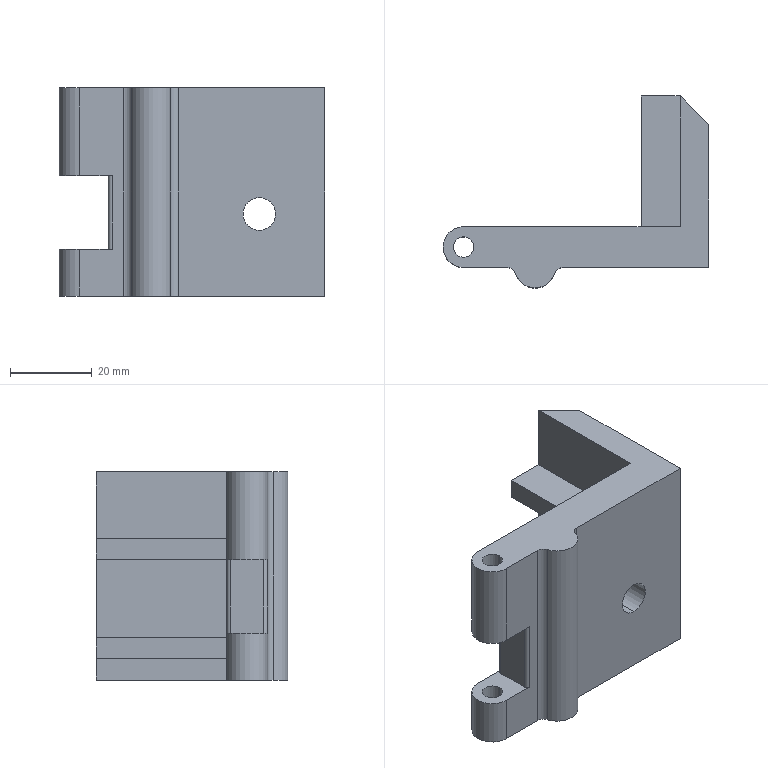Part | Creo | features CURVE 7, PROTRUSION 5, DATUM PLANE 3, ROUND 3, CUT 2, CHAMFER 1, COORDINATE SYSTEM 1 | 1 solid | 34 faces | box 65 x 47 x 51 mm | volume 44748 mm3 | plane 21 | cylinder 13 | commonest cylinder face diameters 5 x4 10 x3 2 x2 4 x2 8 x2
STEP:
#1=CARTESIAN_POINT('',(0.,0.,0.));
#2=DIRECTION('',(0.,0.,1.));
#3=DIRECTION('',(1.,0.,0.));
#4=AXIS2_PLACEMENT_3D('',#1,#2,#3);
#5=CARTESIAN_POINT('',(28.,42.,-20.5));
#6=VERTEX_POINT('',#5);
#7=CARTESIAN_POINT('',(35.,35.,-20.5));
#8=VERTEX_POINT('',#7);
#9=CARTESIAN_POINT('',(28.,42.,-20.5));
#10=DIRECTION('',(0.7071,-0.7071,0.));
#11=VECTOR('',#10,9.899);
#12=LINE('',#9,#11);
#13=EDGE_CURVE('',#6,#8,#12,.T.);
#14=ORIENTED_EDGE('',*,*,#13,.F.);
#15=CARTESIAN_POINT('',(28.,10.,-20.5));
#16=VERTEX_POINT('',#15);
#17=CARTESIAN_POINT('',(28.,42.,-20.5));
#18=DIRECTION('',(0.,-1.,0.));
#19=VECTOR('',#18,32.);
#20=LINE('',#17,#19);
#21=EDGE_CURVE('',#6,#16,#20,.T.);
#22=ORIENTED_EDGE('',*,*,#21,.T.);
#23=CARTESIAN_POINT('',(-25.,10.,-20.5));
#24=VERTEX_POINT('',#23);
#25=CARTESIAN_POINT('',(28.,10.,-20.5));
#26=DIRECTION('',(-1.,0.,0.));
#27=VECTOR('',#26,53.);
#28=LINE('',#25,#27);
#29=EDGE_CURVE('',#16,#24,#28,.T.);
#30=ORIENTED_EDGE('',*,*,#29,.T.);
#31=CARTESIAN_POINT('',(-25.,0.,-20.5));
#32=VERTEX_POINT('',#31);
#33=CARTESIAN_POINT('',(-25.,5.,-20.5));
#34=DIRECTION('',(0.,0.,1.));
#35=DIRECTION('',(0.,1.,0.));
#36=AXIS2_PLACEMENT_3D('',#33,#34,#35);
#37=CIRCLE('',#36,5.);
#38=EDGE_CURVE('',#24,#32,#37,.T.);
#39=ORIENTED_EDGE('',*,*,#38,.T.);
#40=CARTESIAN_POINT('',(-14.208,0.,-20.5));
#41=VERTEX_POINT('',#40);
#42=CARTESIAN_POINT('',(-25.,0.,-20.5));
#43=DIRECTION('',(1.,0.,0.));
#44=VECTOR('',#43,10.792);
#45=LINE('',#42,#44);
#46=EDGE_CURVE('',#32,#41,#45,.T.);
#47=ORIENTED_EDGE('',*,*,#46,.T.);
#48=CARTESIAN_POINT('',(-12.292,-1.429,-20.5));
#49=VERTEX_POINT('',#48);
#50=CARTESIAN_POINT('',(-14.208,-2.,-20.5));
#51=DIRECTION('',(0.,0.,1.));
#52=DIRECTION('',(0.9583,0.2857,0.));
#53=AXIS2_PLACEMENT_3D('',#50,#51,#52);
#54=CIRCLE('',#53,2.);
#55=EDGE_CURVE('',#49,#41,#54,.T.);
#56=ORIENTED_EDGE('',*,*,#55,.F.);
#57=CARTESIAN_POINT('',(-2.708,-1.429,-20.5));
#58=VERTEX_POINT('',#57);
#59=CARTESIAN_POINT('',(-7.5,0.,-20.5));
#60=DIRECTION('',(0.,0.,-1.));
#61=DIRECTION('',(0.9583,-0.2857,0.));
#62=AXIS2_PLACEMENT_3D('',#59,#60,#61);
#63=CIRCLE('',#62,5.);
#64=EDGE_CURVE('',#58,#49,#63,.T.);
#65=ORIENTED_EDGE('',*,*,#64,.F.);
#66=CARTESIAN_POINT('',(-0.7918,0.,-20.5));
#67=VERTEX_POINT('',#66);
#68=CARTESIAN_POINT('',(-0.7918,-2.,-20.5));
#69=DIRECTION('',(0.,0.,1.));
#70=DIRECTION('',(0.,1.,0.));
#71=AXIS2_PLACEMENT_3D('',#68,#69,#70);
#72=CIRCLE('',#71,2.);
#73=EDGE_CURVE('',#67,#58,#72,.T.);
#74=ORIENTED_EDGE('',*,*,#73,.F.);
#75=CARTESIAN_POINT('',(35.,0.,-20.5));
#76=VERTEX_POINT('',#75);
#77=CARTESIAN_POINT('',(35.,0.,-20.5));
#78=DIRECTION('',(-1.,0.,0.));
#79=VECTOR('',#78,35.792);
#80=LINE('',#77,#79);
#81=EDGE_CURVE('',#76,#67,#80,.T.);
#82=ORIENTED_EDGE('',*,*,#81,.F.);
#83=CARTESIAN_POINT('',(35.,0.,-20.5));
#84=DIRECTION('',(0.,1.,0.));
#85=VECTOR('',#84,35.);
#86=LINE('',#83,#85);
#87=EDGE_CURVE('',#76,#8,#86,.T.);
#88=ORIENTED_EDGE('',*,*,#87,.T.);
#89=EDGE_LOOP('',(#14,#22,#30,#39,#47,#56,#65,#74,#82,#88));
#90=FACE_OUTER_BOUND('',#89,.F.);
#91=CARTESIAN_POINT('',(-22.5,5.,-20.5));
#92=VERTEX_POINT('',#91);
#93=CARTESIAN_POINT('',(-27.5,5.,-20.5));
#94=VERTEX_POINT('',#93);
#95=CARTESIAN_POINT('',(-25.,5.,-20.5));
#96=DIRECTION('',(0.,0.,-1.));
#97=DIRECTION('',(1.,0.,0.));
#98=AXIS2_PLACEMENT_3D('',#95,#96,#97);
#99=CIRCLE('',#98,2.5);
#100=EDGE_CURVE('',#92,#94,#99,.T.);
#101=ORIENTED_EDGE('',*,*,#100,.T.);
#102=CARTESIAN_POINT('',(-25.,5.,-20.5));
#103=DIRECTION('',(0.,0.,-1.));
#104=DIRECTION('',(-1.,0.,0.));
#105=AXIS2_PLACEMENT_3D('',#102,#103,#104);
#106=CIRCLE('',#105,2.5);
#107=EDGE_CURVE('',#94,#92,#106,.T.);
#108=ORIENTED_EDGE('',*,*,#107,.T.);
#109=EDGE_LOOP('',(#101,#108));
#110=FACE_BOUND('',#109,.F.);
#111=CARTESIAN_POINT('',(0.,0.,-20.5));
#112=DIRECTION('',(0.,0.,1.));
#113=DIRECTION('',(1.,0.,0.));
#114=AXIS2_PLACEMENT_3D('',#111,#112,#113);
#115=PLANE('',#114);
#116=ADVANCED_FACE('',(#90,#110),#115,.F.);
#117=CARTESIAN_POINT('',(-27.5,5.,-9.));
#118=VERTEX_POINT('',#117);
#119=CARTESIAN_POINT('',(-22.5,5.,-9.));
#120=VERTEX_POINT('',#119);
#121=CARTESIAN_POINT('',(-25.,5.,-9.));
#122=DIRECTION('',(0.,0.,1.));
#123=DIRECTION('',(-1.,0.,0.));
#124=AXIS2_PLACEMENT_3D('',#121,#122,#123);
#125=CIRCLE('',#124,2.5);
#126=EDGE_CURVE('',#118,#120,#125,.T.);
#127=ORIENTED_EDGE('',*,*,#126,.F.);
#128=CARTESIAN_POINT('',(-27.5,5.,-20.5));
#129=DIRECTION('',(0.,0.,1.));
#130=VECTOR('',#129,11.5);
#131=LINE('',#128,#130);
#132=EDGE_CURVE('',#94,#118,#131,.T.);
#133=ORIENTED_EDGE('',*,*,#132,.F.);
#134=ORIENTED_EDGE('',*,*,#100,.F.);
#135=CARTESIAN_POINT('',(-22.5,5.,-20.5));
#136=DIRECTION('',(0.,0.,1.));
#137=VECTOR('',#136,11.5);
#138=LINE('',#135,#137);
#139=EDGE_CURVE('',#92,#120,#138,.T.);
#140=ORIENTED_EDGE('',*,*,#139,.T.);
#141=EDGE_LOOP('',(#127,#133,#134,#140));
#142=FACE_OUTER_BOUND('',#141,.F.);
#143=CARTESIAN_POINT('',(-25.,5.,-20.5));
#144=DIRECTION('',(0.,0.,1.));
#145=DIRECTION('',(1.,0.,0.));
#146=AXIS2_PLACEMENT_3D('',#143,#144,#145);
#147=CYLINDRICAL_SURFACE('',#146,2.5);
#148=ADVANCED_FACE('',(#142),#147,.F.);
#149=CARTESIAN_POINT('',(-22.5,5.,30.5));
#150=VERTEX_POINT('',#149);
#151=CARTESIAN_POINT('',(-22.5,5.,9.));
#152=VERTEX_POINT('',#151);
#153=CARTESIAN_POINT('',(-22.5,5.,30.5));
#154=DIRECTION('',(0.,0.,-1.));
#155=VECTOR('',#154,21.5);
#156=LINE('',#153,#155);
#157=EDGE_CURVE('',#150,#152,#156,.T.);
#158=ORIENTED_EDGE('',*,*,#157,.F.);
#159=CARTESIAN_POINT('',(-27.5,5.,30.5));
#160=VERTEX_POINT('',#159);
#161=CARTESIAN_POINT('',(-25.,5.,30.5));
#162=DIRECTION('',(0.,0.,-1.));
#163=DIRECTION('',(1.,0.,0.));
#164=AXIS2_PLACEMENT_3D('',#161,#162,#163);
#165=CIRCLE('',#164,2.5);
#166=EDGE_CURVE('',#150,#160,#165,.T.);
#167=ORIENTED_EDGE('',*,*,#166,.T.);
#168=CARTESIAN_POINT('',(-27.5,5.,9.));
#169=VERTEX_POINT('',#168);
#170=CARTESIAN_POINT('',(-27.5,5.,9.));
#171=DIRECTION('',(0.,0.,1.));
#172=VECTOR('',#171,21.5);
#173=LINE('',#170,#172);
#174=EDGE_CURVE('',#169,#160,#173,.T.);
#175=ORIENTED_EDGE('',*,*,#174,.F.);
#176=CARTESIAN_POINT('',(-25.,5.,9.));
#177=DIRECTION('',(0.,0.,1.));
#178=DIRECTION('',(-1.,0.,0.));
#179=AXIS2_PLACEMENT_3D('',#176,#177,#178);
#180=CIRCLE('',#179,2.5);
#181=EDGE_CURVE('',#169,#152,#180,.T.);
#182=ORIENTED_EDGE('',*,*,#181,.T.);
#183=EDGE_LOOP('',(#158,#167,#175,#182));
#184=FACE_OUTER_BOUND('',#183,.F.);
#185=CARTESIAN_POINT('',(-25.,5.,-20.5));
#186=DIRECTION('',(0.,0.,1.));
#187=DIRECTION('',(1.,0.,0.));
#188=AXIS2_PLACEMENT_3D('',#185,#186,#187);
#189=CYLINDRICAL_SURFACE('',#188,2.5);
#190=ADVANCED_FACE('',(#184),#189,.F.);
#191=CARTESIAN_POINT('',(-18.,9.,-9.));
#192=VERTEX_POINT('',#191);
#193=CARTESIAN_POINT('',(-18.,1.,-9.));
#194=VERTEX_POINT('',#193);
#195=CARTESIAN_POINT('',(-18.,9.,-9.));
#196=DIRECTION('',(0.,-1.,0.));
#197=VECTOR('',#196,8.);
#198=LINE('',#195,#197);
#199=EDGE_CURVE('',#192,#194,#198,.T.);
#200=ORIENTED_EDGE('',*,*,#199,.T.);
#201=CARTESIAN_POINT('',(-17.,0.,-9.));
#202=VERTEX_POINT('',#201);
#203=CARTESIAN_POINT('',(-17.,1.,-9.));
#204=DIRECTION('',(0.,0.,-1.));
#205=DIRECTION('',(0.,-1.,0.));
#206=AXIS2_PLACEMENT_3D('',#203,#204,#205);
#207=CIRCLE('',#206,1.);
#208=EDGE_CURVE('',#202,#194,#207,.T.);
#209=ORIENTED_EDGE('',*,*,#208,.F.);
#210=CARTESIAN_POINT('',(-25.,0.,-9.));
#211=VERTEX_POINT('',#210);
#212=CARTESIAN_POINT('',(-17.,0.,-9.));
#213=DIRECTION('',(-1.,0.,0.));
#214=VECTOR('',#213,8.);
#215=LINE('',#212,#214);
#216=EDGE_CURVE('',#202,#211,#215,.T.);
#217=ORIENTED_EDGE('',*,*,#216,.T.);
#218=CARTESIAN_POINT('',(-25.,10.,-9.));
#219=VERTEX_POINT('',#218);
#220=CARTESIAN_POINT('',(-25.,5.,-9.));
#221=DIRECTION('',(0.,0.,-1.));
#222=DIRECTION('',(0.,-1.,0.));
#223=AXIS2_PLACEMENT_3D('',#220,#221,#222);
#224=CIRCLE('',#223,5.);
#225=EDGE_CURVE('',#211,#219,#224,.T.);
#226=ORIENTED_EDGE('',*,*,#225,.T.);
#227=CARTESIAN_POINT('',(-17.,10.,-9.));
#228=VERTEX_POINT('',#227);
#229=CARTESIAN_POINT('',(-25.,10.,-9.));
#230=DIRECTION('',(1.,0.,0.));
#231=VECTOR('',#230,8.);
#232=LINE('',#229,#231);
#233=EDGE_CURVE('',#219,#228,#232,.T.);
#234=ORIENTED_EDGE('',*,*,#233,.T.);
#235=CARTESIAN_POINT('',(-17.,9.,-9.));
#236=DIRECTION('',(0.,0.,-1.));
#237=DIRECTION('',(-1.,0.,0.));
#238=AXIS2_PLACEMENT_3D('',#235,#236,#237);
#239=CIRCLE('',#238,1.);
#240=EDGE_CURVE('',#192,#228,#239,.T.);
#241=ORIENTED_EDGE('',*,*,#240,.F.);
#242=EDGE_LOOP('',(#200,#209,#217,#226,#234,#241));
#243=FACE_OUTER_BOUND('',#242,.F.);
#244=ORIENTED_EDGE('',*,*,#126,.T.);
#245=CARTESIAN_POINT('',(-25.,5.,-9.));
#246=DIRECTION('',(0.,0.,1.));
#247=DIRECTION('',(1.,0.,0.));
#248=AXIS2_PLACEMENT_3D('',#245,#246,#247);
#249=CIRCLE('',#248,2.5);
#250=EDGE_CURVE('',#120,#118,#249,.T.);
#251=ORIENTED_EDGE('',*,*,#250,.T.);
#252=EDGE_LOOP('',(#244,#251));
#253=FACE_BOUND('',#252,.F.);
#254=CARTESIAN_POINT('',(-18.,10.,-9.));
#255=DIRECTION('',(0.,0.,-1.));
#256=DIRECTION('',(-1.,0.,0.));
#257=AXIS2_PLACEMENT_3D('',#254,#255,#256);
#258=PLANE('',#257);
#259=ADVANCED_FACE('',(#243,#253),#258,.F.);
#260=ORIENTED_EDGE('',*,*,#250,.F.);
#261=ORIENTED_EDGE('',*,*,#139,.F.);
#262=ORIENTED_EDGE('',*,*,#107,.F.);
#263=ORIENTED_EDGE('',*,*,#132,.T.);
#264=EDGE_LOOP('',(#260,#261,#262,#263));
#265=FACE_OUTER_BOUND('',#264,.F.);
#266=CARTESIAN_POINT('',(-25.,5.,-20.5));
#267=DIRECTION('',(0.,0.,1.));
#268=DIRECTION('',(1.,0.,0.));
#269=AXIS2_PLACEMENT_3D('',#266,#267,#268);
#270=CYLINDRICAL_SURFACE('',#269,2.5);
#271=ADVANCED_FACE('',(#265),#270,.F.);
#272=ORIENTED_EDGE('',*,*,#174,.T.);
#273=CARTESIAN_POINT('',(-25.,5.,30.5));
#274=DIRECTION('',(0.,0.,-1.));
#275=DIRECTION('',(-1.,0.,0.));
#276=AXIS2_PLACEMENT_3D('',#273,#274,#275);
#277=CIRCLE('',#276,2.5);
#278=EDGE_CURVE('',#160,#150,#277,.T.);
#279=ORIENTED_EDGE('',*,*,#278,.T.);
#280=ORIENTED_EDGE('',*,*,#157,.T.);
#281=CARTESIAN_POINT('',(-25.,5.,9.));
#282=DIRECTION('',(0.,0.,1.));
#283=DIRECTION('',(1.,0.,0.));
#284=AXIS2_PLACEMENT_3D('',#281,#282,#283);
#285=CIRCLE('',#284,2.5);
#286=EDGE_CURVE('',#152,#169,#285,.T.);
#287=ORIENTED_EDGE('',*,*,#286,.T.);
#288=EDGE_LOOP('',(#272,#279,#280,#287));
#289=FACE_OUTER_BOUND('',#288,.F.);
#290=CARTESIAN_POINT('',(-25.,5.,-20.5));
#291=DIRECTION('',(0.,0.,1.));
#292=DIRECTION('',(1.,0.,0.));
#293=AXIS2_PLACEMENT_3D('',#290,#291,#292);
#294=CYLINDRICAL_SURFACE('',#293,2.5);
#295=ADVANCED_FACE('',(#289),#294,.F.);
#296=CARTESIAN_POINT('',(35.,35.,30.5));
#297=VERTEX_POINT('',#296);
#298=CARTESIAN_POINT('',(28.,42.,30.5));
#299=VERTEX_POINT('',#298);
#300=CARTESIAN_POINT('',(35.,35.,30.5));
#301=DIRECTION('',(-0.7071,0.7071,0.));
#302=VECTOR('',#301,9.899);
#303=LINE('',#300,#302);
#304=EDGE_CURVE('',#297,#299,#303,.T.);
#305=ORIENTED_EDGE('',*,*,#304,.F.);
#306=CARTESIAN_POINT('',(35.,0.,30.5));
#307=VERTEX_POINT('',#306);
#308=CARTESIAN_POINT('',(35.,35.,30.5));
#309=DIRECTION('',(0.,-1.,0.));
#310=VECTOR('',#309,35.);
#311=LINE('',#308,#310);
#312=EDGE_CURVE('',#297,#307,#311,.T.);
#313=ORIENTED_EDGE('',*,*,#312,.T.);
#314=CARTESIAN_POINT('',(-0.7918,0.,30.5));
#315=VERTEX_POINT('',#314);
#316=CARTESIAN_POINT('',(-0.7918,0.,30.5));
#317=DIRECTION('',(1.,0.,0.));
#318=VECTOR('',#317,35.792);
#319=LINE('',#316,#318);
#320=EDGE_CURVE('',#315,#307,#319,.T.);
#321=ORIENTED_EDGE('',*,*,#320,.F.);
#322=CARTESIAN_POINT('',(-2.708,-1.429,30.5));
#323=VERTEX_POINT('',#322);
#324=CARTESIAN_POINT('',(-0.7918,-2.,30.5));
#325=DIRECTION('',(0.,0.,-1.));
#326=DIRECTION('',(-0.9583,0.2857,0.));
#327=AXIS2_PLACEMENT_3D('',#324,#325,#326);
#328=CIRCLE('',#327,2.);
#329=EDGE_CURVE('',#323,#315,#328,.T.);
#330=ORIENTED_EDGE('',*,*,#329,.F.);
#331=CARTESIAN_POINT('',(-12.292,-1.429,30.5));
#332=VERTEX_POINT('',#331);
#333=CARTESIAN_POINT('',(-7.5,0.,30.5));
#334=DIRECTION('',(0.,0.,1.));
#335=DIRECTION('',(-0.9583,-0.2857,0.));
#336=AXIS2_PLACEMENT_3D('',#333,#334,#335);
#337=CIRCLE('',#336,5.);
#338=EDGE_CURVE('',#332,#323,#337,.T.);
#339=ORIENTED_EDGE('',*,*,#338,.F.);
#340=CARTESIAN_POINT('',(-14.208,0.,30.5));
#341=VERTEX_POINT('',#340);
#342=CARTESIAN_POINT('',(-14.208,-2.,30.5));
#343=DIRECTION('',(0.,0.,-1.));
#344=DIRECTION('',(0.,1.,0.));
#345=AXIS2_PLACEMENT_3D('',#342,#343,#344);
#346=CIRCLE('',#345,2.);
#347=EDGE_CURVE('',#341,#332,#346,.T.);
#348=ORIENTED_EDGE('',*,*,#347,.F.);
#349=CARTESIAN_POINT('',(-25.,0.,30.5));
#350=VERTEX_POINT('',#349);
#351=CARTESIAN_POINT('',(-25.,0.,30.5));
#352=DIRECTION('',(1.,0.,0.));
#353=VECTOR('',#352,10.792);
#354=LINE('',#351,#353);
#355=EDGE_CURVE('',#350,#341,#354,.T.);
#356=ORIENTED_EDGE('',*,*,#355,.F.);
#357=CARTESIAN_POINT('',(-25.,10.,30.5));
#358=VERTEX_POINT('',#357);
#359=CARTESIAN_POINT('',(-25.,5.,30.5));
#360=DIRECTION('',(0.,0.,1.));
#361=DIRECTION('',(0.,1.,0.));
#362=AXIS2_PLACEMENT_3D('',#359,#360,#361);
#363=CIRCLE('',#362,5.);
#364=EDGE_CURVE('',#358,#350,#363,.T.);
#365=ORIENTED_EDGE('',*,*,#364,.F.);
#366=CARTESIAN_POINT('',(28.,10.,30.5));
#367=VERTEX_POINT('',#366);
#368=CARTESIAN_POINT('',(28.,10.,30.5));
#369=DIRECTION('',(-1.,0.,0.));
#370=VECTOR('',#369,53.);
#371=LINE('',#368,#370);
#372=EDGE_CURVE('',#367,#358,#371,.T.);
#373=ORIENTED_EDGE('',*,*,#372,.F.);
#374=CARTESIAN_POINT('',(28.,42.,30.5));
#375=DIRECTION('',(0.,-1.,0.));
#376=VECTOR('',#375,32.);
#377=LINE('',#374,#376);
#378=EDGE_CURVE('',#299,#367,#377,.T.);
#379=ORIENTED_EDGE('',*,*,#378,.F.);
#380=EDGE_LOOP('',(#305,#313,#321,#330,#339,#348,#356,#365,#373,#379));
#381=FACE_OUTER_BOUND('',#380,.F.);
#382=ORIENTED_EDGE('',*,*,#166,.F.);
#383=ORIENTED_EDGE('',*,*,#278,.F.);
#384=EDGE_LOOP('',(#382,#383));
#385=FACE_BOUND('',#384,.F.);
#386=CARTESIAN_POINT('',(0.,0.,30.5));
#387=DIRECTION('',(0.,0.,1.));
#388=DIRECTION('',(1.,0.,0.));
#389=AXIS2_PLACEMENT_3D('',#386,#387,#388);
#390=PLANE('',#389);
#391=ADVANCED_FACE('',(#381,#385),#390,.T.);
#392=ORIENTED_EDGE('',*,*,#304,.T.);
#393=CARTESIAN_POINT('',(28.,42.,14.13));
#394=VERTEX_POINT('',#393);
#395=CARTESIAN_POINT('',(28.,42.,14.13));
#396=DIRECTION('',(0.,0.,1.));
#397=VECTOR('',#396,16.37);
#398=LINE('',#395,#397);
#399=EDGE_CURVE('',#394,#299,#398,.T.);
#400=ORIENTED_EDGE('',*,*,#399,.F.);
#401=CARTESIAN_POINT('',(28.,42.,9.13));
#402=VERTEX_POINT('',#401);
#403=CARTESIAN_POINT('',(28.,42.,9.13));
#404=DIRECTION('',(0.,0.,1.));
#405=VECTOR('',#404,5.);
#406=LINE('',#403,#405);
#407=EDGE_CURVE('',#402,#394,#406,.T.);
#408=ORIENTED_EDGE('',*,*,#407,.F.);
#409=CARTESIAN_POINT('',(28.,42.,-10.13));
#410=VERTEX_POINT('',#409);
#411=CARTESIAN_POINT('',(28.,42.,-10.13));
#412=DIRECTION('',(0.,0.,1.));
#413=VECTOR('',#412,19.26);
#414=LINE('',#411,#413);
#415=EDGE_CURVE('',#410,#402,#414,.T.);
#416=ORIENTED_EDGE('',*,*,#415,.F.);
#417=CARTESIAN_POINT('',(28.,42.,-15.13));
#418=VERTEX_POINT('',#417);
#419=CARTESIAN_POINT('',(28.,42.,-15.13));
#420=DIRECTION('',(0.,0.,1.));
#421=VECTOR('',#420,5.);
#422=LINE('',#419,#421);
#423=EDGE_CURVE('',#418,#410,#422,.T.);
#424=ORIENTED_EDGE('',*,*,#423,.F.);
#425=CARTESIAN_POINT('',(28.,42.,-20.5));
#426=DIRECTION('',(0.,0.,1.));
#427=VECTOR('',#426,5.37);
#428=LINE('',#425,#427);
#429=EDGE_CURVE('',#6,#418,#428,.T.);
#430=ORIENTED_EDGE('',*,*,#429,.F.);
#431=ORIENTED_EDGE('',*,*,#13,.T.);
#432=CARTESIAN_POINT('',(35.,35.,-20.5));
#433=DIRECTION('',(0.,0.,1.));
#434=VECTOR('',#433,51.);
#435=LINE('',#432,#434);
#436=EDGE_CURVE('',#8,#297,#435,.T.);
#437=ORIENTED_EDGE('',*,*,#436,.T.);
#438=EDGE_LOOP('',(#392,#400,#408,#416,#424,#430,#431,#437));
#439=FACE_OUTER_BOUND('',#438,.F.);
#440=CARTESIAN_POINT('',(31.5,38.5,5.));
#441=DIRECTION('',(0.7071,0.7071,0.));
#442=DIRECTION('',(-0.7071,0.7071,0.));
#443=AXIS2_PLACEMENT_3D('',#440,#441,#442);
#444=PLANE('',#443);
#445=ADVANCED_FACE('',(#439),#444,.T.);
#446=ORIENTED_EDGE('',*,*,#399,.T.);
#447=ORIENTED_EDGE('',*,*,#378,.T.);
#448=CARTESIAN_POINT('',(28.,10.,14.13));
#449=VERTEX_POINT('',#448);
#450=CARTESIAN_POINT('',(28.,10.,14.13));
#451=DIRECTION('',(0.,0.,1.));
#452=VECTOR('',#451,16.37);
#453=LINE('',#450,#452);
#454=EDGE_CURVE('',#449,#367,#453,.T.);
#455=ORIENTED_EDGE('',*,*,#454,.F.);
#456=CARTESIAN_POINT('',(28.,42.,14.13));
#457=DIRECTION('',(0.,-1.,0.));
#458=VECTOR('',#457,32.);
#459=LINE('',#456,#458);
#460=EDGE_CURVE('',#394,#449,#459,.T.);
#461=ORIENTED_EDGE('',*,*,#460,.F.);
#462=EDGE_LOOP('',(#446,#447,#455,#461));
#463=FACE_OUTER_BOUND('',#462,.F.);
#464=CARTESIAN_POINT('',(28.,42.,-20.5));
#465=DIRECTION('',(-1.,0.,0.));
#466=DIRECTION('',(0.,-1.,0.));
#467=AXIS2_PLACEMENT_3D('',#464,#465,#466);
#468=PLANE('',#467);
#469=ADVANCED_FACE('',(#463),#468,.T.);
#470=ORIENTED_EDGE('',*,*,#415,.T.);
#471=CARTESIAN_POINT('',(28.,10.,9.13));
#472=VERTEX_POINT('',#471);
#473=CARTESIAN_POINT('',(28.,42.,9.13));
#474=DIRECTION('',(0.,-1.,0.));
#475=VECTOR('',#474,32.);
#476=LINE('',#473,#475);
#477=EDGE_CURVE('',#402,#472,#476,.T.);
#478=ORIENTED_EDGE('',*,*,#477,.T.);
#479=CARTESIAN_POINT('',(28.,10.,-10.13));
#480=VERTEX_POINT('',#479);
#481=CARTESIAN_POINT('',(28.,10.,-10.13));
#482=DIRECTION('',(0.,0.,1.));
#483=VECTOR('',#482,19.26);
#484=LINE('',#481,#483);
#485=EDGE_CURVE('',#480,#472,#484,.T.);
#486=ORIENTED_EDGE('',*,*,#485,.F.);
#487=CARTESIAN_POINT('',(28.,42.,-10.13));
#488=DIRECTION('',(0.,-1.,0.));
#489=VECTOR('',#488,32.);
#490=LINE('',#487,#489);
#491=EDGE_CURVE('',#410,#480,#490,.T.);
#492=ORIENTED_EDGE('',*,*,#491,.F.);
#493=EDGE_LOOP('',(#470,#478,#486,#492));
#494=FACE_OUTER_BOUND('',#493,.F.);
#495=CARTESIAN_POINT('',(28.,42.,-20.5));
#496=DIRECTION('',(-1.,0.,0.));
#497=DIRECTION('',(0.,-1.,0.));
#498=AXIS2_PLACEMENT_3D('',#495,#496,#497);
#499=PLANE('',#498);
#500=ADVANCED_FACE('',(#494),#499,.T.);
#501=ORIENTED_EDGE('',*,*,#429,.T.);
#502=CARTESIAN_POINT('',(28.,10.,-15.13));
#503=VERTEX_POINT('',#502);
#504=CARTESIAN_POINT('',(28.,42.,-15.13));
#505=DIRECTION('',(0.,-1.,0.));
#506=VECTOR('',#505,32.);
#507=LINE('',#504,#506);
#508=EDGE_CURVE('',#418,#503,#507,.T.);
#509=ORIENTED_EDGE('',*,*,#508,.T.);
#510=CARTESIAN_POINT('',(28.,10.,-20.5));
#511=DIRECTION('',(0.,0.,1.));
#512=VECTOR('',#511,5.37);
#513=LINE('',#510,#512);
#514=EDGE_CURVE('',#16,#503,#513,.T.);
#515=ORIENTED_EDGE('',*,*,#514,.F.);
#516=ORIENTED_EDGE('',*,*,#21,.F.);
#517=EDGE_LOOP('',(#501,#509,#515,#516));
#518=FACE_OUTER_BOUND('',#517,.F.);
#519=CARTESIAN_POINT('',(28.,42.,-20.5));
#520=DIRECTION('',(-1.,0.,0.));
#521=DIRECTION('',(0.,-1.,0.));
#522=AXIS2_PLACEMENT_3D('',#519,#520,#521);
#523=PLANE('',#522);
#524=ADVANCED_FACE('',(#518),#523,.T.);
#525=CARTESIAN_POINT('',(18.5,10.,-15.13));
#526=VERTEX_POINT('',#525);
#527=CARTESIAN_POINT('',(28.,10.,-15.13));
#528=DIRECTION('',(-1.,0.,0.));
#529=VECTOR('',#528,9.5);
#530=LINE('',#527,#529);
#531=EDGE_CURVE('',#503,#526,#530,.T.);
#532=ORIENTED_EDGE('',*,*,#531,.T.);
#533=CARTESIAN_POINT('',(18.5,10.,-10.13));
#534=VERTEX_POINT('',#533);
#535=CARTESIAN_POINT('',(18.5,10.,-15.13));
#536=DIRECTION('',(0.,0.,1.));
#537=VECTOR('',#536,5.);
#538=LINE('',#535,#537);
#539=EDGE_CURVE('',#526,#534,#538,.T.);
#540=ORIENTED_EDGE('',*,*,#539,.T.);
#541=CARTESIAN_POINT('',(28.,10.,-10.13));
#542=DIRECTION('',(-1.,0.,0.));
#543=VECTOR('',#542,9.5);
#544=LINE('',#541,#543);
#545=EDGE_CURVE('',#480,#534,#544,.T.);
#546=ORIENTED_EDGE('',*,*,#545,.F.);
#547=ORIENTED_EDGE('',*,*,#485,.T.);
#548=CARTESIAN_POINT('',(18.5,10.,9.13));
#549=VERTEX_POINT('',#548);
#550=CARTESIAN_POINT('',(28.,10.,9.13));
#551=DIRECTION('',(-1.,0.,0.));
#552=VECTOR('',#551,9.5);
#553=LINE('',#550,#552);
#554=EDGE_CURVE('',#472,#549,#553,.T.);
#555=ORIENTED_EDGE('',*,*,#554,.T.);
#556=CARTESIAN_POINT('',(18.5,10.,14.13));
#557=VERTEX_POINT('',#556);
#558=CARTESIAN_POINT('',(18.5,10.,9.13));
#559=DIRECTION('',(0.,0.,1.));
#560=VECTOR('',#559,5.);
#561=LINE('',#558,#560);
#562=EDGE_CURVE('',#549,#557,#561,.T.);
#563=ORIENTED_EDGE('',*,*,#562,.T.);
#564=CARTESIAN_POINT('',(28.,10.,14.13));
#565=DIRECTION('',(-1.,0.,0.));
#566=VECTOR('',#565,9.5);
#567=LINE('',#564,#566);
#568=EDGE_CURVE('',#449,#557,#567,.T.);
#569=ORIENTED_EDGE('',*,*,#568,.F.);
#570=ORIENTED_EDGE('',*,*,#454,.T.);
#571=ORIENTED_EDGE('',*,*,#372,.T.);
#572=CARTESIAN_POINT('',(-25.,10.,9.));
#573=VERTEX_POINT('',#572);
#574=CARTESIAN_POINT('',(-25.,10.,30.5));
#575=DIRECTION('',(0.,0.,-1.));
#576=VECTOR('',#575,21.5);
#577=LINE('',#574,#576);
#578=EDGE_CURVE('',#358,#573,#577,.T.);
#579=ORIENTED_EDGE('',*,*,#578,.T.);
#580=CARTESIAN_POINT('',(-17.,10.,9.));
#581=VERTEX_POINT('',#580);
#582=CARTESIAN_POINT('',(-17.,10.,9.));
#583=DIRECTION('',(-1.,0.,0.));
#584=VECTOR('',#583,8.);
#585=LINE('',#582,#584);
#586=EDGE_CURVE('',#581,#573,#585,.T.);
#587=ORIENTED_EDGE('',*,*,#586,.F.);
#588=CARTESIAN_POINT('',(-17.,10.,-9.));
#589=DIRECTION('',(0.,0.,1.));
#590=VECTOR('',#589,18.);
#591=LINE('',#588,#590);
#592=EDGE_CURVE('',#228,#581,#591,.T.);
#593=ORIENTED_EDGE('',*,*,#592,.F.);
#594=ORIENTED_EDGE('',*,*,#233,.F.);
#595=CARTESIAN_POINT('',(-25.,10.,-9.));
#596=DIRECTION('',(0.,0.,-1.));
#597=VECTOR('',#596,11.5);
#598=LINE('',#595,#597);
#599=EDGE_CURVE('',#219,#24,#598,.T.);
#600=ORIENTED_EDGE('',*,*,#599,.T.);
#601=ORIENTED_EDGE('',*,*,#29,.F.);
#602=ORIENTED_EDGE('',*,*,#514,.T.);
#603=EDGE_LOOP('',(#532,#540,#546,#547,#555,#563,#569,#570,#571,#579,#587,#593,#594,#600,#601,#602));
#604=FACE_OUTER_BOUND('',#603,.F.);
#605=CARTESIAN_POINT('',(19.,10.,-4.39));
#606=VERTEX_POINT('',#605);
#607=CARTESIAN_POINT('',(19.,10.,3.61));
#608=VERTEX_POINT('',#607);
#609=CARTESIAN_POINT('',(19.,10.,-0.3895));
#610=DIRECTION('',(0.,1.,0.));
#611=DIRECTION('',(0.,0.,-1.));
#612=AXIS2_PLACEMENT_3D('',#609,#610,#611);
#613=CIRCLE('',#612,4.);
#614=EDGE_CURVE('',#606,#608,#613,.T.);
#615=ORIENTED_EDGE('',*,*,#614,.T.);
#616=CARTESIAN_POINT('',(19.,10.,-0.3895));
#617=DIRECTION('',(0.,1.,0.));
#618=DIRECTION('',(0.,0.,1.));
#619=AXIS2_PLACEMENT_3D('',#616,#617,#618);
#620=CIRCLE('',#619,4.);
#621=EDGE_CURVE('',#608,#606,#620,.T.);
#622=ORIENTED_EDGE('',*,*,#621,.T.);
#623=EDGE_LOOP('',(#615,#622));
#624=FACE_BOUND('',#623,.F.);
#625=CARTESIAN_POINT('',(28.,10.,-20.5));
#626=DIRECTION('',(0.,1.,0.));
#627=DIRECTION('',(-1.,0.,0.));
#628=AXIS2_PLACEMENT_3D('',#625,#626,#627);
#629=PLANE('',#628);
#630=ADVANCED_FACE('',(#604,#624),#629,.T.);
#631=ORIENTED_EDGE('',*,*,#508,.F.);
#632=CARTESIAN_POINT('',(18.5,42.,-15.13));
#633=VERTEX_POINT('',#632);
#634=CARTESIAN_POINT('',(28.,42.,-15.13));
#635=DIRECTION('',(-1.,0.,0.));
#636=VECTOR('',#635,9.5);
#637=LINE('',#634,#636);
#638=EDGE_CURVE('',#418,#633,#637,.T.);
#639=ORIENTED_EDGE('',*,*,#638,.T.);
#640=CARTESIAN_POINT('',(18.5,10.,-15.13));
#641=DIRECTION('',(0.,1.,0.));
#642=VECTOR('',#641,32.);
#643=LINE('',#640,#642);
#644=EDGE_CURVE('',#526,#633,#643,.T.);
#645=ORIENTED_EDGE('',*,*,#644,.F.);
#646=ORIENTED_EDGE('',*,*,#531,.F.);
#647=EDGE_LOOP('',(#631,#639,#645,#646));
#648=FACE_OUTER_BOUND('',#647,.F.);
#649=CARTESIAN_POINT('',(28.,10.,-15.13));
#650=DIRECTION('',(0.,0.,-1.));
#651=DIRECTION('',(-1.,0.,0.));
#652=AXIS2_PLACEMENT_3D('',#649,#650,#651);
#653=PLANE('',#652);
#654=ADVANCED_FACE('',(#648),#653,.T.);
#655=ORIENTED_EDGE('',*,*,#407,.T.);
#656=CARTESIAN_POINT('',(18.5,42.,14.13));
#657=VERTEX_POINT('',#656);
#658=CARTESIAN_POINT('',(18.5,42.,14.13));
#659=DIRECTION('',(1.,0.,0.));
#660=VECTOR('',#659,9.5);
#661=LINE('',#658,#660);
#662=EDGE_CURVE('',#657,#394,#661,.T.);
#663=ORIENTED_EDGE('',*,*,#662,.F.);
#664=CARTESIAN_POINT('',(18.5,42.,9.13));
#665=VERTEX_POINT('',#664);
#666=CARTESIAN_POINT('',(18.5,42.,9.13));
#667=DIRECTION('',(0.,0.,1.));
#668=VECTOR('',#667,5.);
#669=LINE('',#666,#668);
#670=EDGE_CURVE('',#665,#657,#669,.T.);
#671=ORIENTED_EDGE('',*,*,#670,.F.);
#672=CARTESIAN_POINT('',(28.,42.,9.13));
#673=DIRECTION('',(-1.,0.,0.));
#674=VECTOR('',#673,9.5);
#675=LINE('',#672,#674);
#676=EDGE_CURVE('',#402,#665,#675,.T.);
#677=ORIENTED_EDGE('',*,*,#676,.F.);
#678=EDGE_LOOP('',(#655,#663,#671,#677));
#679=FACE_OUTER_BOUND('',#678,.F.);
#680=CARTESIAN_POINT('',(30.,42.,-20.5));
#681=DIRECTION('',(0.,1.,0.));
#682=DIRECTION('',(-1.,0.,0.));
#683=AXIS2_PLACEMENT_3D('',#680,#681,#682);
#684=PLANE('',#683);
#685=ADVANCED_FACE('',(#679),#684,.T.);
#686=ORIENTED_EDGE('',*,*,#423,.T.);
#687=CARTESIAN_POINT('',(18.5,42.,-10.13));
#688=VERTEX_POINT('',#687);
#689=CARTESIAN_POINT('',(18.5,42.,-10.13));
#690=DIRECTION('',(1.,0.,0.));
#691=VECTOR('',#690,9.5);
#692=LINE('',#689,#691);
#693=EDGE_CURVE('',#688,#410,#692,.T.);
#694=ORIENTED_EDGE('',*,*,#693,.F.);
#695=CARTESIAN_POINT('',(18.5,42.,-15.13));
#696=DIRECTION('',(0.,0.,1.));
#697=VECTOR('',#696,5.);
#698=LINE('',#695,#697);
#699=EDGE_CURVE('',#633,#688,#698,.T.);
#700=ORIENTED_EDGE('',*,*,#699,.F.);
#701=ORIENTED_EDGE('',*,*,#638,.F.);
#702=EDGE_LOOP('',(#686,#694,#700,#701));
#703=FACE_OUTER_BOUND('',#702,.F.);
#704=CARTESIAN_POINT('',(30.,42.,-20.5));
#705=DIRECTION('',(0.,1.,0.));
#706=DIRECTION('',(-1.,0.,0.));
#707=AXIS2_PLACEMENT_3D('',#704,#705,#706);
#708=PLANE('',#707);
#709=ADVANCED_FACE('',(#703),#708,.T.);
#710=ORIENTED_EDGE('',*,*,#460,.T.);
#711=ORIENTED_EDGE('',*,*,#568,.T.);
#712=CARTESIAN_POINT('',(18.5,10.,14.13));
#713=DIRECTION('',(0.,1.,0.));
#714=VECTOR('',#713,32.);
#715=LINE('',#712,#714);
#716=EDGE_CURVE('',#557,#657,#715,.T.);
#717=ORIENTED_EDGE('',*,*,#716,.T.);
#718=ORIENTED_EDGE('',*,*,#662,.T.);
#719=EDGE_LOOP('',(#710,#711,#717,#718));
#720=FACE_OUTER_BOUND('',#719,.F.);
#721=CARTESIAN_POINT('',(18.5,10.,14.13));
#722=DIRECTION('',(0.,0.,1.));
#723=DIRECTION('',(1.,0.,0.));
#724=AXIS2_PLACEMENT_3D('',#721,#722,#723);
#725=PLANE('',#724);
#726=ADVANCED_FACE('',(#720),#725,.T.);
#727=ORIENTED_EDGE('',*,*,#562,.F.);
#728=CARTESIAN_POINT('',(18.5,10.,9.13));
#729=DIRECTION('',(0.,1.,0.));
#730=VECTOR('',#729,32.);
#731=LINE('',#728,#730);
#732=EDGE_CURVE('',#549,#665,#731,.T.);
#733=ORIENTED_EDGE('',*,*,#732,.T.);
#734=ORIENTED_EDGE('',*,*,#670,.T.);
#735=ORIENTED_EDGE('',*,*,#716,.F.);
#736=EDGE_LOOP('',(#727,#733,#734,#735));
#737=FACE_OUTER_BOUND('',#736,.F.);
#738=CARTESIAN_POINT('',(18.5,10.,9.13));
#739=DIRECTION('',(-1.,0.,0.));
#740=DIRECTION('',(0.,0.,1.));
#741=AXIS2_PLACEMENT_3D('',#738,#739,#740);
#742=PLANE('',#741);
#743=ADVANCED_FACE('',(#737),#742,.T.);
#744=ORIENTED_EDGE('',*,*,#477,.F.);
#745=ORIENTED_EDGE('',*,*,#676,.T.);
#746=ORIENTED_EDGE('',*,*,#732,.F.);
#747=ORIENTED_EDGE('',*,*,#554,.F.);
#748=EDGE_LOOP('',(#744,#745,#746,#747));
#749=FACE_OUTER_BOUND('',#748,.F.);
#750=CARTESIAN_POINT('',(28.,10.,9.13));
#751=DIRECTION('',(0.,0.,-1.));
#752=DIRECTION('',(-1.,0.,0.));
#753=AXIS2_PLACEMENT_3D('',#750,#751,#752);
#754=PLANE('',#753);
#755=ADVANCED_FACE('',(#749),#754,.T.);
#756=ORIENTED_EDGE('',*,*,#491,.T.);
#757=ORIENTED_EDGE('',*,*,#545,.T.);
#758=CARTESIAN_POINT('',(18.5,10.,-10.13));
#759=DIRECTION('',(0.,1.,0.));
#760=VECTOR('',#759,32.);
#761=LINE('',#758,#760);
#762=EDGE_CURVE('',#534,#688,#761,.T.);
#763=ORIENTED_EDGE('',*,*,#762,.T.);
#764=ORIENTED_EDGE('',*,*,#693,.T.);
#765=EDGE_LOOP('',(#756,#757,#763,#764));
#766=FACE_OUTER_BOUND('',#765,.F.);
#767=CARTESIAN_POINT('',(18.5,10.,-10.13));
#768=DIRECTION('',(0.,0.,1.));
#769=DIRECTION('',(1.,0.,0.));
#770=AXIS2_PLACEMENT_3D('',#767,#768,#769);
#771=PLANE('',#770);
#772=ADVANCED_FACE('',(#766),#771,.T.);
#773=ORIENTED_EDGE('',*,*,#539,.F.);
#774=ORIENTED_EDGE('',*,*,#644,.T.);
#775=ORIENTED_EDGE('',*,*,#699,.T.);
#776=ORIENTED_EDGE('',*,*,#762,.F.);
#777=EDGE_LOOP('',(#773,#774,#775,#776));
#778=FACE_OUTER_BOUND('',#777,.F.);
#779=CARTESIAN_POINT('',(18.5,10.,-15.13));
#780=DIRECTION('',(-1.,0.,0.));
#781=DIRECTION('',(0.,0.,1.));
#782=AXIS2_PLACEMENT_3D('',#779,#780,#781);
#783=PLANE('',#782);
#784=ADVANCED_FACE('',(#778),#783,.T.);
#785=ORIENTED_EDGE('',*,*,#578,.F.);
#786=ORIENTED_EDGE('',*,*,#364,.T.);
#787=CARTESIAN_POINT('',(-25.,0.,9.));
#788=VERTEX_POINT('',#787);
#789=CARTESIAN_POINT('',(-25.,0.,9.));
#790=DIRECTION('',(0.,0.,1.));
#791=VECTOR('',#790,21.5);
#792=LINE('',#789,#791);
#793=EDGE_CURVE('',#788,#350,#792,.T.);
#794=ORIENTED_EDGE('',*,*,#793,.F.);
#795=CARTESIAN_POINT('',(-25.,5.,9.));
#796=DIRECTION('',(0.,0.,1.));
#797=DIRECTION('',(0.,1.,0.));
#798=AXIS2_PLACEMENT_3D('',#795,#796,#797);
#799=CIRCLE('',#798,5.);
#800=EDGE_CURVE('',#573,#788,#799,.T.);
#801=ORIENTED_EDGE('',*,*,#800,.F.);
#802=EDGE_LOOP('',(#785,#786,#794,#801));
#803=FACE_OUTER_BOUND('',#802,.F.);
#804=CARTESIAN_POINT('',(-25.,5.,73.948));
#805=DIRECTION('',(0.,0.,-1.));
#806=DIRECTION('',(-1.,0.,0.));
#807=AXIS2_PLACEMENT_3D('',#804,#805,#806);
#808=CYLINDRICAL_SURFACE('',#807,5.);
#809=ADVANCED_FACE('',(#803),#808,.T.);
#810=ORIENTED_EDGE('',*,*,#793,.T.);
#811=ORIENTED_EDGE('',*,*,#355,.T.);
#812=CARTESIAN_POINT('',(-14.208,0.,-20.5));
#813=DIRECTION('',(0.,0.,1.));
#814=VECTOR('',#813,51.);
#815=LINE('',#812,#814);
#816=EDGE_CURVE('',#41,#341,#815,.T.);
#817=ORIENTED_EDGE('',*,*,#816,.F.);
#818=ORIENTED_EDGE('',*,*,#46,.F.);
#819=CARTESIAN_POINT('',(-25.,0.,-9.));
#820=DIRECTION('',(0.,0.,-1.));
#821=VECTOR('',#820,11.5);
#822=LINE('',#819,#821);
#823=EDGE_CURVE('',#211,#32,#822,.T.);
#824=ORIENTED_EDGE('',*,*,#823,.F.);
#825=ORIENTED_EDGE('',*,*,#216,.F.);
#826=CARTESIAN_POINT('',(-17.,0.,9.));
#827=VERTEX_POINT('',#826);
#828=CARTESIAN_POINT('',(-17.,0.,9.));
#829=DIRECTION('',(0.,0.,-1.));
#830=VECTOR('',#829,18.);
#831=LINE('',#828,#830);
#832=EDGE_CURVE('',#827,#202,#831,.T.);
#833=ORIENTED_EDGE('',*,*,#832,.F.);
#834=CARTESIAN_POINT('',(-25.,0.,9.));
#835=DIRECTION('',(1.,0.,0.));
#836=VECTOR('',#835,8.);
#837=LINE('',#834,#836);
#838=EDGE_CURVE('',#788,#827,#837,.T.);
#839=ORIENTED_EDGE('',*,*,#838,.F.);
#840=EDGE_LOOP('',(#810,#811,#817,#818,#824,#825,#833,#839));
#841=FACE_OUTER_BOUND('',#840,.F.);
#842=CARTESIAN_POINT('',(-30.,0.,-20.5));
#843=DIRECTION('',(0.,-1.,0.));
#844=DIRECTION('',(1.,0.,0.));
#845=AXIS2_PLACEMENT_3D('',#842,#843,#844);
#846=PLANE('',#845);
#847=ADVANCED_FACE('',(#841),#846,.T.);
#848=ORIENTED_EDGE('',*,*,#320,.T.);
#849=CARTESIAN_POINT('',(35.,0.,30.5));
#850=DIRECTION('',(0.,0.,-1.));
#851=VECTOR('',#850,51.);
#852=LINE('',#849,#851);
#853=EDGE_CURVE('',#307,#76,#852,.T.);
#854=ORIENTED_EDGE('',*,*,#853,.T.);
#855=ORIENTED_EDGE('',*,*,#81,.T.);
#856=CARTESIAN_POINT('',(-0.7918,0.,30.5));
#857=DIRECTION('',(0.,0.,-1.));
#858=VECTOR('',#857,51.);
#859=LINE('',#856,#858);
#860=EDGE_CURVE('',#315,#67,#859,.T.);
#861=ORIENTED_EDGE('',*,*,#860,.F.);
#862=EDGE_LOOP('',(#848,#854,#855,#861));
#863=FACE_OUTER_BOUND('',#862,.F.);
#864=CARTESIAN_POINT('',(19.,0.,-4.39));
#865=VERTEX_POINT('',#864);
#866=CARTESIAN_POINT('',(19.,0.,3.61));
#867=VERTEX_POINT('',#866);
#868=CARTESIAN_POINT('',(19.,0.,-0.3895));
#869=DIRECTION('',(0.,1.,0.));
#870=DIRECTION('',(0.,0.,-1.));
#871=AXIS2_PLACEMENT_3D('',#868,#869,#870);
#872=CIRCLE('',#871,4.);
#873=EDGE_CURVE('',#865,#867,#872,.T.);
#874=ORIENTED_EDGE('',*,*,#873,.F.);
#875=CARTESIAN_POINT('',(19.,0.,-0.3895));
#876=DIRECTION('',(0.,1.,0.));
#877=DIRECTION('',(0.,0.,1.));
#878=AXIS2_PLACEMENT_3D('',#875,#876,#877);
#879=CIRCLE('',#878,4.);
#880=EDGE_CURVE('',#867,#865,#879,.T.);
#881=ORIENTED_EDGE('',*,*,#880,.F.);
#882=EDGE_LOOP('',(#874,#881));
#883=FACE_BOUND('',#882,.F.);
#884=CARTESIAN_POINT('',(-30.,0.,-20.5));
#885=DIRECTION('',(0.,-1.,0.));
#886=DIRECTION('',(1.,0.,0.));
#887=AXIS2_PLACEMENT_3D('',#884,#885,#886);
#888=PLANE('',#887);
#889=ADVANCED_FACE('',(#863,#883),#888,.T.);
#890=ORIENTED_EDGE('',*,*,#816,.T.);
#891=ORIENTED_EDGE('',*,*,#347,.T.);
#892=CARTESIAN_POINT('',(-12.292,-1.429,-20.5));
#893=DIRECTION('',(0.,0.,1.));
#894=VECTOR('',#893,51.);
#895=LINE('',#892,#894);
#896=EDGE_CURVE('',#49,#332,#895,.T.);
#897=ORIENTED_EDGE('',*,*,#896,.F.);
#898=ORIENTED_EDGE('',*,*,#55,.T.);
#899=EDGE_LOOP('',(#890,#891,#897,#898));
#900=FACE_OUTER_BOUND('',#899,.F.);
#901=CARTESIAN_POINT('',(-14.208,-2.,73.948));
#902=DIRECTION('',(0.,0.,-1.));
#903=DIRECTION('',(0.,1.,0.));
#904=AXIS2_PLACEMENT_3D('',#901,#902,#903);
#905=CYLINDRICAL_SURFACE('',#904,2.);
#906=ADVANCED_FACE('',(#900),#905,.F.);
#907=ORIENTED_EDGE('',*,*,#896,.T.);
#908=ORIENTED_EDGE('',*,*,#338,.T.);
#909=CARTESIAN_POINT('',(-2.708,-1.429,-20.5));
#910=DIRECTION('',(0.,0.,1.));
#911=VECTOR('',#910,51.);
#912=LINE('',#909,#911);
#913=EDGE_CURVE('',#58,#323,#912,.T.);
#914=ORIENTED_EDGE('',*,*,#913,.F.);
#915=ORIENTED_EDGE('',*,*,#64,.T.);
#916=EDGE_LOOP('',(#907,#908,#914,#915));
#917=FACE_OUTER_BOUND('',#916,.F.);
#918=CARTESIAN_POINT('',(-7.5,0.,20.5));
#919=DIRECTION('',(0.,0.,1.));
#920=DIRECTION('',(0.,1.,0.));
#921=AXIS2_PLACEMENT_3D('',#918,#919,#920);
#922=CYLINDRICAL_SURFACE('',#921,5.);
#923=ADVANCED_FACE('',(#917),#922,.T.);
#924=ORIENTED_EDGE('',*,*,#913,.T.);
#925=ORIENTED_EDGE('',*,*,#329,.T.);
#926=ORIENTED_EDGE('',*,*,#860,.T.);
#927=ORIENTED_EDGE('',*,*,#73,.T.);
#928=EDGE_LOOP('',(#924,#925,#926,#927));
#929=FACE_OUTER_BOUND('',#928,.F.);
#930=CARTESIAN_POINT('',(-0.7918,-2.,-73.948));
#931=DIRECTION('',(0.,0.,1.));
#932=DIRECTION('',(0.,1.,0.));
#933=AXIS2_PLACEMENT_3D('',#930,#931,#932);
#934=CYLINDRICAL_SURFACE('',#933,2.);
#935=ADVANCED_FACE('',(#929),#934,.F.);
#936=ORIENTED_EDGE('',*,*,#38,.F.);
#937=ORIENTED_EDGE('',*,*,#599,.F.);
#938=ORIENTED_EDGE('',*,*,#225,.F.);
#939=ORIENTED_EDGE('',*,*,#823,.T.);
#940=EDGE_LOOP('',(#936,#937,#938,#939));
#941=FACE_OUTER_BOUND('',#940,.F.);
#942=CARTESIAN_POINT('',(-25.,5.,73.948));
#943=DIRECTION('',(0.,0.,-1.));
#944=DIRECTION('',(0.,-1.,0.));
#945=AXIS2_PLACEMENT_3D('',#942,#943,#944);
#946=CYLINDRICAL_SURFACE('',#945,5.);
#947=ADVANCED_FACE('',(#941),#946,.T.);
#948=CARTESIAN_POINT('',(-18.,1.,9.));
#949=VERTEX_POINT('',#948);
#950=CARTESIAN_POINT('',(-18.,1.,9.));
#951=DIRECTION('',(0.,0.,-1.));
#952=VECTOR('',#951,18.);
#953=LINE('',#950,#952);
#954=EDGE_CURVE('',#949,#194,#953,.T.);
#955=ORIENTED_EDGE('',*,*,#954,.F.);
#956=CARTESIAN_POINT('',(-17.,1.,9.));
#957=DIRECTION('',(0.,0.,1.));
#958=DIRECTION('',(-1.,0.,0.));
#959=AXIS2_PLACEMENT_3D('',#956,#957,#958);
#960=CIRCLE('',#959,1.);
#961=EDGE_CURVE('',#949,#827,#960,.T.);
#962=ORIENTED_EDGE('',*,*,#961,.T.);
#963=ORIENTED_EDGE('',*,*,#832,.T.);
#964=ORIENTED_EDGE('',*,*,#208,.T.);
#965=EDGE_LOOP('',(#955,#962,#963,#964));
#966=FACE_OUTER_BOUND('',#965,.F.);
#967=CARTESIAN_POINT('',(-17.,1.,73.948));
#968=DIRECTION('',(0.,0.,-1.));
#969=DIRECTION('',(0.,-1.,0.));
#970=AXIS2_PLACEMENT_3D('',#967,#968,#969);
#971=CYLINDRICAL_SURFACE('',#970,1.);
#972=ADVANCED_FACE('',(#966),#971,.T.);
#973=CARTESIAN_POINT('',(-18.,9.,9.));
#974=VERTEX_POINT('',#973);
#975=CARTESIAN_POINT('',(-18.,9.,-9.));
#976=DIRECTION('',(0.,0.,1.));
#977=VECTOR('',#976,18.);
#978=LINE('',#975,#977);
#979=EDGE_CURVE('',#192,#974,#978,.T.);
#980=ORIENTED_EDGE('',*,*,#979,.T.);
#981=CARTESIAN_POINT('',(-18.,9.,9.));
#982=DIRECTION('',(0.,-1.,0.));
#983=VECTOR('',#982,8.);
#984=LINE('',#981,#983);
#985=EDGE_CURVE('',#974,#949,#984,.T.);
#986=ORIENTED_EDGE('',*,*,#985,.T.);
#987=ORIENTED_EDGE('',*,*,#954,.T.);
#988=ORIENTED_EDGE('',*,*,#199,.F.);
#989=EDGE_LOOP('',(#980,#986,#987,#988));
#990=FACE_OUTER_BOUND('',#989,.F.);
#991=CARTESIAN_POINT('',(-18.,10.,9.));
#992=DIRECTION('',(1.,0.,0.));
#993=DIRECTION('',(0.,0.,-1.));
#994=AXIS2_PLACEMENT_3D('',#991,#992,#993);
#995=PLANE('',#994);
#996=ADVANCED_FACE('',(#990),#995,.F.);
#997=ORIENTED_EDGE('',*,*,#979,.F.);
#998=ORIENTED_EDGE('',*,*,#240,.T.);
#999=ORIENTED_EDGE('',*,*,#592,.T.);
#1000=CARTESIAN_POINT('',(-17.,9.,9.));
#1001=DIRECTION('',(0.,0.,1.));
#1002=DIRECTION('',(0.,1.,0.));
#1003=AXIS2_PLACEMENT_3D('',#1000,#1001,#1002);
#1004=CIRCLE('',#1003,1.);
#1005=EDGE_CURVE('',#581,#974,#1004,.T.);
#1006=ORIENTED_EDGE('',*,*,#1005,.T.);
#1007=EDGE_LOOP('',(#997,#998,#999,#1006));
#1008=FACE_OUTER_BOUND('',#1007,.F.);
#1009=CARTESIAN_POINT('',(-17.,9.,-73.948));
#1010=DIRECTION('',(0.,0.,1.));
#1011=DIRECTION('',(0.,1.,0.));
#1012=AXIS2_PLACEMENT_3D('',#1009,#1010,#1011);
#1013=CYLINDRICAL_SURFACE('',#1012,1.);
#1014=ADVANCED_FACE('',(#1008),#1013,.T.);
#1015=ORIENTED_EDGE('',*,*,#838,.T.);
#1016=ORIENTED_EDGE('',*,*,#961,.F.);
#1017=ORIENTED_EDGE('',*,*,#985,.F.);
#1018=ORIENTED_EDGE('',*,*,#1005,.F.);
#1019=ORIENTED_EDGE('',*,*,#586,.T.);
#1020=ORIENTED_EDGE('',*,*,#800,.T.);
#1021=EDGE_LOOP('',(#1015,#1016,#1017,#1018,#1019,#1020));
#1022=FACE_OUTER_BOUND('',#1021,.F.);
#1023=ORIENTED_EDGE('',*,*,#181,.F.);
#1024=ORIENTED_EDGE('',*,*,#286,.F.);
#1025=EDGE_LOOP('',(#1023,#1024));
#1026=FACE_BOUND('',#1025,.F.);
#1027=CARTESIAN_POINT('',(-30.,10.,9.));
#1028=DIRECTION('',(0.,0.,1.));
#1029=DIRECTION('',(1.,0.,0.));
#1030=AXIS2_PLACEMENT_3D('',#1027,#1028,#1029);
#1031=PLANE('',#1030);
#1032=ADVANCED_FACE('',(#1022,#1026),#1031,.F.);
#1033=ORIENTED_EDGE('',*,*,#436,.F.);
#1034=ORIENTED_EDGE('',*,*,#87,.F.);
#1035=ORIENTED_EDGE('',*,*,#853,.F.);
#1036=ORIENTED_EDGE('',*,*,#312,.F.);
#1037=EDGE_LOOP('',(#1033,#1034,#1035,#1036));
#1038=FACE_OUTER_BOUND('',#1037,.F.);
#1039=CARTESIAN_POINT('',(35.,0.,-20.5));
#1040=DIRECTION('',(1.,0.,0.));
#1041=DIRECTION('',(0.,0.,-1.));
#1042=AXIS2_PLACEMENT_3D('',#1039,#1040,#1041);
#1043=PLANE('',#1042);
#1044=ADVANCED_FACE('',(#1038),#1043,.T.);
#1045=ORIENTED_EDGE('',*,*,#614,.F.);
#1046=CARTESIAN_POINT('',(19.,10.,-4.39));
#1047=DIRECTION('',(0.,-1.,0.));
#1048=VECTOR('',#1047,10.);
#1049=LINE('',#1046,#1048);
#1050=EDGE_CURVE('',#606,#865,#1049,.T.);
#1051=ORIENTED_EDGE('',*,*,#1050,.T.);
#1052=ORIENTED_EDGE('',*,*,#873,.T.);
#1053=CARTESIAN_POINT('',(19.,10.,3.61));
#1054=DIRECTION('',(0.,-1.,0.));
#1055=VECTOR('',#1054,10.);
#1056=LINE('',#1053,#1055);
#1057=EDGE_CURVE('',#608,#867,#1056,.T.);
#1058=ORIENTED_EDGE('',*,*,#1057,.F.);
#1059=EDGE_LOOP('',(#1045,#1051,#1052,#1058));
#1060=FACE_OUTER_BOUND('',#1059,.F.);
#1061=CARTESIAN_POINT('',(19.,10.,-0.3895));
#1062=DIRECTION('',(0.,1.,0.));
#1063=DIRECTION('',(0.,0.,-1.));
#1064=AXIS2_PLACEMENT_3D('',#1061,#1062,#1063);
#1065=CYLINDRICAL_SURFACE('',#1064,4.);
#1066=ADVANCED_FACE('',(#1060),#1065,.F.);
#1067=ORIENTED_EDGE('',*,*,#621,.F.);
#1068=ORIENTED_EDGE('',*,*,#1057,.T.);
#1069=ORIENTED_EDGE('',*,*,#880,.T.);
#1070=ORIENTED_EDGE('',*,*,#1050,.F.);
#1071=EDGE_LOOP('',(#1067,#1068,#1069,#1070));
#1072=FACE_OUTER_BOUND('',#1071,.F.);
#1073=CARTESIAN_POINT('',(19.,10.,-0.3895));
#1074=DIRECTION('',(0.,1.,0.));
#1075=DIRECTION('',(0.,0.,-1.));
#1076=AXIS2_PLACEMENT_3D('',#1073,#1074,#1075);
#1077=CYLINDRICAL_SURFACE('',#1076,4.);
#1078=ADVANCED_FACE('',(#1072),#1077,.F.);
#1079=CLOSED_SHELL('',(#116,#148,#190,#259,#271,#295,#391,#445,#469,#500,#524,#630,#654,#685,#709,#726,#743,#755,#772,#784,#809,#847,#889,#906,#923,#935,#947,#972,#996,#1014,#1032,#1044,#1066,#1078));
#1080=MANIFOLD_SOLID_BREP('',#1079);
#1081=(LENGTH_UNIT()NAMED_UNIT(*)SI_UNIT(.MILLI.,.METRE.));
#1082=UNCERTAINTY_MEASURE_WITH_UNIT(LENGTH_MEASURE(0.009506),#1081,'','');
#1083=(NAMED_UNIT(*)PLANE_ANGLE_UNIT()SI_UNIT($,.RADIAN.));
#1084=PLANE_ANGLE_MEASURE_WITH_UNIT(PLANE_ANGLE_MEASURE(0.01745),#1083);
#1085=(CONVERSION_BASED_UNIT('DEGREE',#1084)NAMED_UNIT(*)PLANE_ANGLE_UNIT());
#1086=(NAMED_UNIT(*)SI_UNIT($,.STERADIAN.)SOLID_ANGLE_UNIT());
#1087=(GEOMETRIC_REPRESENTATION_CONTEXT(3)GLOBAL_UNCERTAINTY_ASSIGNED_CONTEXT((#1082))GLOBAL_UNIT_ASSIGNED_CONTEXT((#1081,#1085,#1086))REPRESENTATION_CONTEXT('',''));
#1088=ADVANCED_BREP_SHAPE_REPRESENTATION('',(#4,#1080),#1087);